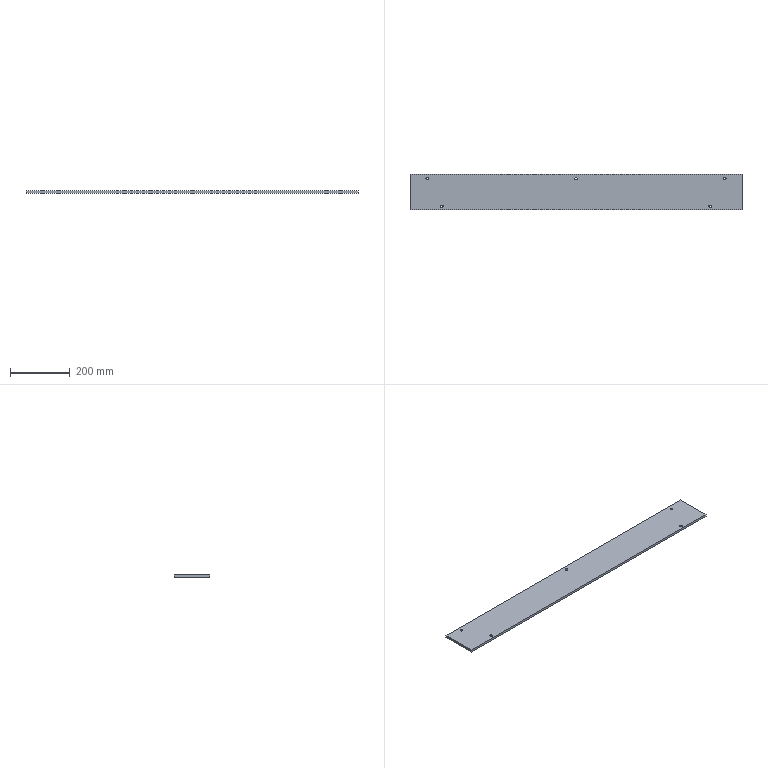Part | SolidWorks | features Extrusion 1, HoleWzd 1 | 1 solid | 16 faces | box 1116 x 120 x 8 mm | volume 1069090 mm3 | cylinder 10 | plane 6 | commonest cylinder face diameters 8.5 x10
STEP:
#1=CARTESIAN_POINT('',(-504.25,45.,0.));
#2=VERTEX_POINT('',#1);
#3=CARTESIAN_POINT('',(-495.75,45.,0.));
#4=VERTEX_POINT('',#3);
#5=CARTESIAN_POINT('',(-500.,45.,0.));
#6=DIRECTION('',(0.,0.,1.));
#7=DIRECTION('',(1.,0.,0.));
#8=AXIS2_PLACEMENT_3D('',#5,#6,#7);
#9=CIRCLE('',#8,4.25);
#10=EDGE_CURVE('',#2,#4,#9,.T.);
#11=ORIENTED_EDGE('',*,*,#10,.F.);
#12=CARTESIAN_POINT('',(-504.25,45.,8.));
#13=VERTEX_POINT('',#12);
#14=CARTESIAN_POINT('',(-504.25,45.,8.));
#15=DIRECTION('',(0.,0.,1.));
#16=VECTOR('',#15,1000.);
#17=LINE('',#14,#16);
#18=EDGE_CURVE('',#2,#13,#17,.T.);
#19=ORIENTED_EDGE('',*,*,#18,.T.);
#20=CARTESIAN_POINT('',(-495.75,45.,8.));
#21=VERTEX_POINT('',#20);
#22=CARTESIAN_POINT('',(-500.,45.,8.));
#23=DIRECTION('',(0.,0.,1.));
#24=DIRECTION('',(1.,0.,0.));
#25=AXIS2_PLACEMENT_3D('',#22,#23,#24);
#26=CIRCLE('',#25,4.25);
#27=EDGE_CURVE('',#13,#21,#26,.T.);
#28=ORIENTED_EDGE('',*,*,#27,.T.);
#29=CARTESIAN_POINT('',(-495.75,45.,8.));
#30=DIRECTION('',(0.,0.,1.));
#31=VECTOR('',#30,1000.);
#32=LINE('',#29,#31);
#33=EDGE_CURVE('',#4,#21,#32,.T.);
#34=ORIENTED_EDGE('',*,*,#33,.F.);
#35=EDGE_LOOP('',(#11,#19,#28,#34));
#36=FACE_OUTER_BOUND('',#35,.T.);
#37=CARTESIAN_POINT('',(-500.,45.,8.));
#38=DIRECTION('',(0.,0.,1.));
#39=DIRECTION('',(1.,0.,0.));
#40=AXIS2_PLACEMENT_3D('',#37,#38,#39);
#41=CYLINDRICAL_SURFACE('',#40,4.25);
#42=ADVANCED_FACE('',(#36),#41,.F.);
#43=CARTESIAN_POINT('',(-455.25,-48.,0.));
#44=VERTEX_POINT('',#43);
#45=CARTESIAN_POINT('',(-446.75,-48.,0.));
#46=VERTEX_POINT('',#45);
#47=CARTESIAN_POINT('',(-451.,-48.,0.));
#48=DIRECTION('',(0.,0.,1.));
#49=DIRECTION('',(1.,0.,0.));
#50=AXIS2_PLACEMENT_3D('',#47,#48,#49);
#51=CIRCLE('',#50,4.25);
#52=EDGE_CURVE('',#44,#46,#51,.T.);
#53=ORIENTED_EDGE('',*,*,#52,.F.);
#54=CARTESIAN_POINT('',(-455.25,-48.,8.));
#55=VERTEX_POINT('',#54);
#56=CARTESIAN_POINT('',(-455.25,-48.,8.));
#57=DIRECTION('',(0.,0.,1.));
#58=VECTOR('',#57,1000.);
#59=LINE('',#56,#58);
#60=EDGE_CURVE('',#44,#55,#59,.T.);
#61=ORIENTED_EDGE('',*,*,#60,.T.);
#62=CARTESIAN_POINT('',(-446.75,-48.,8.));
#63=VERTEX_POINT('',#62);
#64=CARTESIAN_POINT('',(-451.,-48.,8.));
#65=DIRECTION('',(0.,0.,1.));
#66=DIRECTION('',(1.,0.,0.));
#67=AXIS2_PLACEMENT_3D('',#64,#65,#66);
#68=CIRCLE('',#67,4.25);
#69=EDGE_CURVE('',#55,#63,#68,.T.);
#70=ORIENTED_EDGE('',*,*,#69,.T.);
#71=CARTESIAN_POINT('',(-446.75,-48.,8.));
#72=DIRECTION('',(0.,0.,1.));
#73=VECTOR('',#72,1000.);
#74=LINE('',#71,#73);
#75=EDGE_CURVE('',#46,#63,#74,.T.);
#76=ORIENTED_EDGE('',*,*,#75,.F.);
#77=EDGE_LOOP('',(#53,#61,#70,#76));
#78=FACE_OUTER_BOUND('',#77,.T.);
#79=CARTESIAN_POINT('',(-451.,-48.,8.));
#80=DIRECTION('',(0.,0.,1.));
#81=DIRECTION('',(1.,0.,0.));
#82=AXIS2_PLACEMENT_3D('',#79,#80,#81);
#83=CYLINDRICAL_SURFACE('',#82,4.25);
#84=ADVANCED_FACE('',(#78),#83,.F.);
#85=CARTESIAN_POINT('',(-4.25,45.,0.));
#86=VERTEX_POINT('',#85);
#87=CARTESIAN_POINT('',(4.25,45.,0.));
#88=VERTEX_POINT('',#87);
#89=CARTESIAN_POINT('',(0.,45.,0.));
#90=DIRECTION('',(0.,0.,1.));
#91=DIRECTION('',(1.,0.,0.));
#92=AXIS2_PLACEMENT_3D('',#89,#90,#91);
#93=CIRCLE('',#92,4.25);
#94=EDGE_CURVE('',#86,#88,#93,.T.);
#95=ORIENTED_EDGE('',*,*,#94,.F.);
#96=CARTESIAN_POINT('',(-4.25,45.,8.));
#97=VERTEX_POINT('',#96);
#98=CARTESIAN_POINT('',(-4.25,45.,8.));
#99=DIRECTION('',(0.,0.,1.));
#100=VECTOR('',#99,1000.);
#101=LINE('',#98,#100);
#102=EDGE_CURVE('',#86,#97,#101,.T.);
#103=ORIENTED_EDGE('',*,*,#102,.T.);
#104=CARTESIAN_POINT('',(4.25,45.,8.));
#105=VERTEX_POINT('',#104);
#106=CARTESIAN_POINT('',(0.,45.,8.));
#107=DIRECTION('',(0.,0.,1.));
#108=DIRECTION('',(1.,0.,0.));
#109=AXIS2_PLACEMENT_3D('',#106,#107,#108);
#110=CIRCLE('',#109,4.25);
#111=EDGE_CURVE('',#97,#105,#110,.T.);
#112=ORIENTED_EDGE('',*,*,#111,.T.);
#113=CARTESIAN_POINT('',(4.25,45.,8.));
#114=DIRECTION('',(0.,0.,1.));
#115=VECTOR('',#114,1000.);
#116=LINE('',#113,#115);
#117=EDGE_CURVE('',#88,#105,#116,.T.);
#118=ORIENTED_EDGE('',*,*,#117,.F.);
#119=EDGE_LOOP('',(#95,#103,#112,#118));
#120=FACE_OUTER_BOUND('',#119,.T.);
#121=CARTESIAN_POINT('',(0.,45.,8.));
#122=DIRECTION('',(0.,0.,1.));
#123=DIRECTION('',(1.,0.,0.));
#124=AXIS2_PLACEMENT_3D('',#121,#122,#123);
#125=CYLINDRICAL_SURFACE('',#124,4.25);
#126=ADVANCED_FACE('',(#120),#125,.F.);
#127=CARTESIAN_POINT('',(495.75,45.,0.));
#128=VERTEX_POINT('',#127);
#129=CARTESIAN_POINT('',(504.25,45.,0.));
#130=VERTEX_POINT('',#129);
#131=CARTESIAN_POINT('',(500.,45.,0.));
#132=DIRECTION('',(0.,0.,1.));
#133=DIRECTION('',(1.,0.,0.));
#134=AXIS2_PLACEMENT_3D('',#131,#132,#133);
#135=CIRCLE('',#134,4.25);
#136=EDGE_CURVE('',#128,#130,#135,.T.);
#137=ORIENTED_EDGE('',*,*,#136,.F.);
#138=CARTESIAN_POINT('',(495.75,45.,8.));
#139=VERTEX_POINT('',#138);
#140=CARTESIAN_POINT('',(495.75,45.,8.));
#141=DIRECTION('',(0.,0.,1.));
#142=VECTOR('',#141,1000.);
#143=LINE('',#140,#142);
#144=EDGE_CURVE('',#128,#139,#143,.T.);
#145=ORIENTED_EDGE('',*,*,#144,.T.);
#146=CARTESIAN_POINT('',(504.25,45.,8.));
#147=VERTEX_POINT('',#146);
#148=CARTESIAN_POINT('',(500.,45.,8.));
#149=DIRECTION('',(0.,0.,1.));
#150=DIRECTION('',(1.,0.,0.));
#151=AXIS2_PLACEMENT_3D('',#148,#149,#150);
#152=CIRCLE('',#151,4.25);
#153=EDGE_CURVE('',#139,#147,#152,.T.);
#154=ORIENTED_EDGE('',*,*,#153,.T.);
#155=CARTESIAN_POINT('',(504.25,45.,8.));
#156=DIRECTION('',(0.,0.,1.));
#157=VECTOR('',#156,1000.);
#158=LINE('',#155,#157);
#159=EDGE_CURVE('',#130,#147,#158,.T.);
#160=ORIENTED_EDGE('',*,*,#159,.F.);
#161=EDGE_LOOP('',(#137,#145,#154,#160));
#162=FACE_OUTER_BOUND('',#161,.T.);
#163=CARTESIAN_POINT('',(500.,45.,8.));
#164=DIRECTION('',(0.,0.,1.));
#165=DIRECTION('',(1.,0.,0.));
#166=AXIS2_PLACEMENT_3D('',#163,#164,#165);
#167=CYLINDRICAL_SURFACE('',#166,4.25);
#168=ADVANCED_FACE('',(#162),#167,.F.);
#169=CARTESIAN_POINT('',(446.75,-48.,0.));
#170=VERTEX_POINT('',#169);
#171=CARTESIAN_POINT('',(455.25,-48.,0.));
#172=VERTEX_POINT('',#171);
#173=CARTESIAN_POINT('',(451.,-48.,0.));
#174=DIRECTION('',(0.,0.,1.));
#175=DIRECTION('',(1.,0.,0.));
#176=AXIS2_PLACEMENT_3D('',#173,#174,#175);
#177=CIRCLE('',#176,4.25);
#178=EDGE_CURVE('',#170,#172,#177,.T.);
#179=ORIENTED_EDGE('',*,*,#178,.F.);
#180=CARTESIAN_POINT('',(446.75,-48.,8.));
#181=VERTEX_POINT('',#180);
#182=CARTESIAN_POINT('',(446.75,-48.,8.));
#183=DIRECTION('',(0.,0.,1.));
#184=VECTOR('',#183,1000.);
#185=LINE('',#182,#184);
#186=EDGE_CURVE('',#170,#181,#185,.T.);
#187=ORIENTED_EDGE('',*,*,#186,.T.);
#188=CARTESIAN_POINT('',(455.25,-48.,8.));
#189=VERTEX_POINT('',#188);
#190=CARTESIAN_POINT('',(451.,-48.,8.));
#191=DIRECTION('',(0.,0.,1.));
#192=DIRECTION('',(1.,0.,0.));
#193=AXIS2_PLACEMENT_3D('',#190,#191,#192);
#194=CIRCLE('',#193,4.25);
#195=EDGE_CURVE('',#181,#189,#194,.T.);
#196=ORIENTED_EDGE('',*,*,#195,.T.);
#197=CARTESIAN_POINT('',(455.25,-48.,8.));
#198=DIRECTION('',(0.,0.,1.));
#199=VECTOR('',#198,1000.);
#200=LINE('',#197,#199);
#201=EDGE_CURVE('',#172,#189,#200,.T.);
#202=ORIENTED_EDGE('',*,*,#201,.F.);
#203=EDGE_LOOP('',(#179,#187,#196,#202));
#204=FACE_OUTER_BOUND('',#203,.T.);
#205=CARTESIAN_POINT('',(451.,-48.,8.));
#206=DIRECTION('',(0.,0.,1.));
#207=DIRECTION('',(1.,0.,0.));
#208=AXIS2_PLACEMENT_3D('',#205,#206,#207);
#209=CYLINDRICAL_SURFACE('',#208,4.25);
#210=ADVANCED_FACE('',(#204),#209,.F.);
#211=CARTESIAN_POINT('',(558.,-60.,0.));
#212=VERTEX_POINT('',#211);
#213=CARTESIAN_POINT('',(558.,60.,0.));
#214=VERTEX_POINT('',#213);
#215=CARTESIAN_POINT('',(558.,60.,0.));
#216=DIRECTION('',(0.,1.,0.));
#217=VECTOR('',#216,1000.);
#218=LINE('',#215,#217);
#219=EDGE_CURVE('',#212,#214,#218,.T.);
#220=ORIENTED_EDGE('',*,*,#219,.T.);
#221=CARTESIAN_POINT('',(558.,60.,8.));
#222=VERTEX_POINT('',#221);
#223=CARTESIAN_POINT('',(558.,60.,8.));
#224=DIRECTION('',(0.,0.,-1.));
#225=VECTOR('',#224,1000.);
#226=LINE('',#223,#225);
#227=EDGE_CURVE('',#222,#214,#226,.T.);
#228=ORIENTED_EDGE('',*,*,#227,.F.);
#229=CARTESIAN_POINT('',(558.,-60.,8.));
#230=VERTEX_POINT('',#229);
#231=CARTESIAN_POINT('',(558.,60.,8.));
#232=DIRECTION('',(0.,1.,0.));
#233=VECTOR('',#232,1000.);
#234=LINE('',#231,#233);
#235=EDGE_CURVE('',#230,#222,#234,.T.);
#236=ORIENTED_EDGE('',*,*,#235,.F.);
#237=CARTESIAN_POINT('',(558.,-60.,8.));
#238=DIRECTION('',(0.,0.,-1.));
#239=VECTOR('',#238,1000.);
#240=LINE('',#237,#239);
#241=EDGE_CURVE('',#230,#212,#240,.T.);
#242=ORIENTED_EDGE('',*,*,#241,.T.);
#243=EDGE_LOOP('',(#220,#228,#236,#242));
#244=FACE_OUTER_BOUND('',#243,.T.);
#245=CARTESIAN_POINT('',(558.,60.,8.));
#246=DIRECTION('',(-1.,0.,0.));
#247=DIRECTION('',(0.,0.,1.));
#248=AXIS2_PLACEMENT_3D('',#245,#246,#247);
#249=PLANE('',#248);
#250=ADVANCED_FACE('',(#244),#249,.F.);
#251=CARTESIAN_POINT('',(-558.,60.,0.));
#252=VERTEX_POINT('',#251);
#253=CARTESIAN_POINT('',(-558.,60.,0.));
#254=DIRECTION('',(-1.,0.,0.));
#255=VECTOR('',#254,1000.);
#256=LINE('',#253,#255);
#257=EDGE_CURVE('',#214,#252,#256,.T.);
#258=ORIENTED_EDGE('',*,*,#257,.T.);
#259=CARTESIAN_POINT('',(-558.,60.,8.));
#260=VERTEX_POINT('',#259);
#261=CARTESIAN_POINT('',(-558.,60.,8.));
#262=DIRECTION('',(0.,0.,-1.));
#263=VECTOR('',#262,1000.);
#264=LINE('',#261,#263);
#265=EDGE_CURVE('',#260,#252,#264,.T.);
#266=ORIENTED_EDGE('',*,*,#265,.F.);
#267=CARTESIAN_POINT('',(-558.,60.,8.));
#268=DIRECTION('',(-1.,0.,0.));
#269=VECTOR('',#268,1000.);
#270=LINE('',#267,#269);
#271=EDGE_CURVE('',#222,#260,#270,.T.);
#272=ORIENTED_EDGE('',*,*,#271,.F.);
#273=ORIENTED_EDGE('',*,*,#227,.T.);
#274=EDGE_LOOP('',(#258,#266,#272,#273));
#275=FACE_OUTER_BOUND('',#274,.T.);
#276=CARTESIAN_POINT('',(-558.,60.,8.));
#277=DIRECTION('',(0.,-1.,0.));
#278=DIRECTION('',(0.,0.,-1.));
#279=AXIS2_PLACEMENT_3D('',#276,#277,#278);
#280=PLANE('',#279);
#281=ADVANCED_FACE('',(#275),#280,.F.);
#282=CARTESIAN_POINT('',(-558.,-60.,0.));
#283=VERTEX_POINT('',#282);
#284=CARTESIAN_POINT('',(-558.,60.,0.));
#285=DIRECTION('',(0.,-1.,0.));
#286=VECTOR('',#285,1000.);
#287=LINE('',#284,#286);
#288=EDGE_CURVE('',#252,#283,#287,.T.);
#289=ORIENTED_EDGE('',*,*,#288,.T.);
#290=CARTESIAN_POINT('',(-558.,-60.,8.));
#291=VERTEX_POINT('',#290);
#292=CARTESIAN_POINT('',(-558.,-60.,8.));
#293=DIRECTION('',(0.,0.,-1.));
#294=VECTOR('',#293,1000.);
#295=LINE('',#292,#294);
#296=EDGE_CURVE('',#291,#283,#295,.T.);
#297=ORIENTED_EDGE('',*,*,#296,.F.);
#298=CARTESIAN_POINT('',(-558.,60.,8.));
#299=DIRECTION('',(0.,-1.,0.));
#300=VECTOR('',#299,1000.);
#301=LINE('',#298,#300);
#302=EDGE_CURVE('',#260,#291,#301,.T.);
#303=ORIENTED_EDGE('',*,*,#302,.F.);
#304=ORIENTED_EDGE('',*,*,#265,.T.);
#305=EDGE_LOOP('',(#289,#297,#303,#304));
#306=FACE_OUTER_BOUND('',#305,.T.);
#307=CARTESIAN_POINT('',(-558.,60.,8.));
#308=DIRECTION('',(1.,0.,0.));
#309=DIRECTION('',(0.,0.,-1.));
#310=AXIS2_PLACEMENT_3D('',#307,#308,#309);
#311=PLANE('',#310);
#312=ADVANCED_FACE('',(#306),#311,.F.);
#313=CARTESIAN_POINT('',(-558.,-60.,0.));
#314=DIRECTION('',(1.,0.,0.));
#315=VECTOR('',#314,1000.);
#316=LINE('',#313,#315);
#317=EDGE_CURVE('',#283,#212,#316,.T.);
#318=ORIENTED_EDGE('',*,*,#317,.T.);
#319=ORIENTED_EDGE('',*,*,#241,.F.);
#320=CARTESIAN_POINT('',(-558.,-60.,8.));
#321=DIRECTION('',(1.,0.,0.));
#322=VECTOR('',#321,1000.);
#323=LINE('',#320,#322);
#324=EDGE_CURVE('',#291,#230,#323,.T.);
#325=ORIENTED_EDGE('',*,*,#324,.F.);
#326=ORIENTED_EDGE('',*,*,#296,.T.);
#327=EDGE_LOOP('',(#318,#319,#325,#326));
#328=FACE_OUTER_BOUND('',#327,.T.);
#329=CARTESIAN_POINT('',(-558.,-60.,8.));
#330=DIRECTION('',(0.,1.,0.));
#331=DIRECTION('',(0.,0.,1.));
#332=AXIS2_PLACEMENT_3D('',#329,#330,#331);
#333=PLANE('',#332);
#334=ADVANCED_FACE('',(#328),#333,.F.);
#335=CARTESIAN_POINT('',(-500.,45.,8.));
#336=DIRECTION('',(0.,0.,1.));
#337=DIRECTION('',(1.,0.,0.));
#338=AXIS2_PLACEMENT_3D('',#335,#336,#337);
#339=CIRCLE('',#338,4.25);
#340=EDGE_CURVE('',#21,#13,#339,.T.);
#341=ORIENTED_EDGE('',*,*,#340,.F.);
#342=ORIENTED_EDGE('',*,*,#27,.F.);
#343=EDGE_LOOP('',(#341,#342));
#344=FACE_BOUND('',#343,.T.);
#345=CARTESIAN_POINT('',(-451.,-48.,8.));
#346=DIRECTION('',(0.,0.,1.));
#347=DIRECTION('',(1.,0.,0.));
#348=AXIS2_PLACEMENT_3D('',#345,#346,#347);
#349=CIRCLE('',#348,4.25);
#350=EDGE_CURVE('',#63,#55,#349,.T.);
#351=ORIENTED_EDGE('',*,*,#350,.F.);
#352=ORIENTED_EDGE('',*,*,#69,.F.);
#353=EDGE_LOOP('',(#351,#352));
#354=FACE_BOUND('',#353,.T.);
#355=CARTESIAN_POINT('',(0.,45.,8.));
#356=DIRECTION('',(0.,0.,1.));
#357=DIRECTION('',(1.,0.,0.));
#358=AXIS2_PLACEMENT_3D('',#355,#356,#357);
#359=CIRCLE('',#358,4.25);
#360=EDGE_CURVE('',#105,#97,#359,.T.);
#361=ORIENTED_EDGE('',*,*,#360,.F.);
#362=ORIENTED_EDGE('',*,*,#111,.F.);
#363=EDGE_LOOP('',(#361,#362));
#364=FACE_BOUND('',#363,.T.);
#365=CARTESIAN_POINT('',(500.,45.,8.));
#366=DIRECTION('',(0.,0.,1.));
#367=DIRECTION('',(1.,0.,0.));
#368=AXIS2_PLACEMENT_3D('',#365,#366,#367);
#369=CIRCLE('',#368,4.25);
#370=EDGE_CURVE('',#147,#139,#369,.T.);
#371=ORIENTED_EDGE('',*,*,#370,.F.);
#372=ORIENTED_EDGE('',*,*,#153,.F.);
#373=EDGE_LOOP('',(#371,#372));
#374=FACE_BOUND('',#373,.T.);
#375=CARTESIAN_POINT('',(451.,-48.,8.));
#376=DIRECTION('',(0.,0.,1.));
#377=DIRECTION('',(1.,0.,0.));
#378=AXIS2_PLACEMENT_3D('',#375,#376,#377);
#379=CIRCLE('',#378,4.25);
#380=EDGE_CURVE('',#189,#181,#379,.T.);
#381=ORIENTED_EDGE('',*,*,#380,.F.);
#382=ORIENTED_EDGE('',*,*,#195,.F.);
#383=EDGE_LOOP('',(#381,#382));
#384=FACE_BOUND('',#383,.T.);
#385=ORIENTED_EDGE('',*,*,#235,.T.);
#386=ORIENTED_EDGE('',*,*,#271,.T.);
#387=ORIENTED_EDGE('',*,*,#302,.T.);
#388=ORIENTED_EDGE('',*,*,#324,.T.);
#389=EDGE_LOOP('',(#385,#386,#387,#388));
#390=FACE_OUTER_BOUND('',#389,.T.);
#391=CARTESIAN_POINT('',(0.,0.,8.));
#392=DIRECTION('',(0.,0.,1.));
#393=DIRECTION('',(1.,0.,0.));
#394=AXIS2_PLACEMENT_3D('',#391,#392,#393);
#395=PLANE('',#394);
#396=ADVANCED_FACE('',(#344,#354,#364,#374,#384,#390),#395,.T.);
#397=CARTESIAN_POINT('',(-500.,45.,0.));
#398=DIRECTION('',(0.,0.,1.));
#399=DIRECTION('',(1.,0.,0.));
#400=AXIS2_PLACEMENT_3D('',#397,#398,#399);
#401=CIRCLE('',#400,4.25);
#402=EDGE_CURVE('',#4,#2,#401,.T.);
#403=ORIENTED_EDGE('',*,*,#402,.T.);
#404=ORIENTED_EDGE('',*,*,#10,.T.);
#405=EDGE_LOOP('',(#403,#404));
#406=FACE_BOUND('',#405,.T.);
#407=CARTESIAN_POINT('',(-451.,-48.,0.));
#408=DIRECTION('',(0.,0.,1.));
#409=DIRECTION('',(1.,0.,0.));
#410=AXIS2_PLACEMENT_3D('',#407,#408,#409);
#411=CIRCLE('',#410,4.25);
#412=EDGE_CURVE('',#46,#44,#411,.T.);
#413=ORIENTED_EDGE('',*,*,#412,.T.);
#414=ORIENTED_EDGE('',*,*,#52,.T.);
#415=EDGE_LOOP('',(#413,#414));
#416=FACE_BOUND('',#415,.T.);
#417=CARTESIAN_POINT('',(0.,45.,0.));
#418=DIRECTION('',(0.,0.,1.));
#419=DIRECTION('',(1.,0.,0.));
#420=AXIS2_PLACEMENT_3D('',#417,#418,#419);
#421=CIRCLE('',#420,4.25);
#422=EDGE_CURVE('',#88,#86,#421,.T.);
#423=ORIENTED_EDGE('',*,*,#422,.T.);
#424=ORIENTED_EDGE('',*,*,#94,.T.);
#425=EDGE_LOOP('',(#423,#424));
#426=FACE_BOUND('',#425,.T.);
#427=CARTESIAN_POINT('',(500.,45.,0.));
#428=DIRECTION('',(0.,0.,1.));
#429=DIRECTION('',(1.,0.,0.));
#430=AXIS2_PLACEMENT_3D('',#427,#428,#429);
#431=CIRCLE('',#430,4.25);
#432=EDGE_CURVE('',#130,#128,#431,.T.);
#433=ORIENTED_EDGE('',*,*,#432,.T.);
#434=ORIENTED_EDGE('',*,*,#136,.T.);
#435=EDGE_LOOP('',(#433,#434));
#436=FACE_BOUND('',#435,.T.);
#437=CARTESIAN_POINT('',(451.,-48.,0.));
#438=DIRECTION('',(0.,0.,1.));
#439=DIRECTION('',(1.,0.,0.));
#440=AXIS2_PLACEMENT_3D('',#437,#438,#439);
#441=CIRCLE('',#440,4.25);
#442=EDGE_CURVE('',#172,#170,#441,.T.);
#443=ORIENTED_EDGE('',*,*,#442,.T.);
#444=ORIENTED_EDGE('',*,*,#178,.T.);
#445=EDGE_LOOP('',(#443,#444));
#446=FACE_BOUND('',#445,.T.);
#447=ORIENTED_EDGE('',*,*,#219,.F.);
#448=ORIENTED_EDGE('',*,*,#317,.F.);
#449=ORIENTED_EDGE('',*,*,#288,.F.);
#450=ORIENTED_EDGE('',*,*,#257,.F.);
#451=EDGE_LOOP('',(#447,#448,#449,#450));
#452=FACE_OUTER_BOUND('',#451,.T.);
#453=CARTESIAN_POINT('',(0.,0.,0.));
#454=DIRECTION('',(0.,0.,1.));
#455=DIRECTION('',(1.,0.,0.));
#456=AXIS2_PLACEMENT_3D('',#453,#454,#455);
#457=PLANE('',#456);
#458=ADVANCED_FACE('',(#406,#416,#426,#436,#446,#452),#457,.F.);
#459=ORIENTED_EDGE('',*,*,#186,.F.);
#460=ORIENTED_EDGE('',*,*,#442,.F.);
#461=ORIENTED_EDGE('',*,*,#201,.T.);
#462=ORIENTED_EDGE('',*,*,#380,.T.);
#463=EDGE_LOOP('',(#459,#460,#461,#462));
#464=FACE_OUTER_BOUND('',#463,.T.);
#465=CARTESIAN_POINT('',(451.,-48.,8.));
#466=DIRECTION('',(0.,0.,1.));
#467=DIRECTION('',(1.,0.,0.));
#468=AXIS2_PLACEMENT_3D('',#465,#466,#467);
#469=CYLINDRICAL_SURFACE('',#468,4.25);
#470=ADVANCED_FACE('',(#464),#469,.F.);
#471=ORIENTED_EDGE('',*,*,#144,.F.);
#472=ORIENTED_EDGE('',*,*,#432,.F.);
#473=ORIENTED_EDGE('',*,*,#159,.T.);
#474=ORIENTED_EDGE('',*,*,#370,.T.);
#475=EDGE_LOOP('',(#471,#472,#473,#474));
#476=FACE_OUTER_BOUND('',#475,.T.);
#477=CARTESIAN_POINT('',(500.,45.,8.));
#478=DIRECTION('',(0.,0.,1.));
#479=DIRECTION('',(1.,0.,0.));
#480=AXIS2_PLACEMENT_3D('',#477,#478,#479);
#481=CYLINDRICAL_SURFACE('',#480,4.25);
#482=ADVANCED_FACE('',(#476),#481,.F.);
#483=ORIENTED_EDGE('',*,*,#102,.F.);
#484=ORIENTED_EDGE('',*,*,#422,.F.);
#485=ORIENTED_EDGE('',*,*,#117,.T.);
#486=ORIENTED_EDGE('',*,*,#360,.T.);
#487=EDGE_LOOP('',(#483,#484,#485,#486));
#488=FACE_OUTER_BOUND('',#487,.T.);
#489=CARTESIAN_POINT('',(0.,45.,8.));
#490=DIRECTION('',(0.,0.,1.));
#491=DIRECTION('',(1.,0.,0.));
#492=AXIS2_PLACEMENT_3D('',#489,#490,#491);
#493=CYLINDRICAL_SURFACE('',#492,4.25);
#494=ADVANCED_FACE('',(#488),#493,.F.);
#495=ORIENTED_EDGE('',*,*,#60,.F.);
#496=ORIENTED_EDGE('',*,*,#412,.F.);
#497=ORIENTED_EDGE('',*,*,#75,.T.);
#498=ORIENTED_EDGE('',*,*,#350,.T.);
#499=EDGE_LOOP('',(#495,#496,#497,#498));
#500=FACE_OUTER_BOUND('',#499,.T.);
#501=CARTESIAN_POINT('',(-451.,-48.,8.));
#502=DIRECTION('',(0.,0.,1.));
#503=DIRECTION('',(1.,0.,0.));
#504=AXIS2_PLACEMENT_3D('',#501,#502,#503);
#505=CYLINDRICAL_SURFACE('',#504,4.25);
#506=ADVANCED_FACE('',(#500),#505,.F.);
#507=ORIENTED_EDGE('',*,*,#18,.F.);
#508=ORIENTED_EDGE('',*,*,#402,.F.);
#509=ORIENTED_EDGE('',*,*,#33,.T.);
#510=ORIENTED_EDGE('',*,*,#340,.T.);
#511=EDGE_LOOP('',(#507,#508,#509,#510));
#512=FACE_OUTER_BOUND('',#511,.T.);
#513=CARTESIAN_POINT('',(-500.,45.,8.));
#514=DIRECTION('',(0.,0.,1.));
#515=DIRECTION('',(1.,0.,0.));
#516=AXIS2_PLACEMENT_3D('',#513,#514,#515);
#517=CYLINDRICAL_SURFACE('',#516,4.25);
#518=ADVANCED_FACE('',(#512),#517,.F.);
#519=CLOSED_SHELL('',(#42,#84,#126,#168,#210,#250,#281,#312,#334,#396,#458,#470,#482,#494,#506,#518));
#520=MANIFOLD_SOLID_BREP('',#519);
#521=CARTESIAN_POINT('',(0.,0.,0.));
#522=DIRECTION('',(0.,0.,1.));
#523=DIRECTION('',(1.,0.,0.));
#524=AXIS2_PLACEMENT_3D('',#521,#522,#523);
#525=(LENGTH_UNIT()NAMED_UNIT(*)SI_UNIT(.MILLI.,.METRE.));
#526=UNCERTAINTY_MEASURE_WITH_UNIT(LENGTH_MEASURE(0.00001),#525,'','');
#527=(NAMED_UNIT(*)PLANE_ANGLE_UNIT()SI_UNIT($,.RADIAN.));
#528=(NAMED_UNIT(*)SI_UNIT($,.STERADIAN.)SOLID_ANGLE_UNIT());
#529=(GEOMETRIC_REPRESENTATION_CONTEXT(3)GLOBAL_UNCERTAINTY_ASSIGNED_CONTEXT((#526))GLOBAL_UNIT_ASSIGNED_CONTEXT((#525,#527,#528))REPRESENTATION_CONTEXT('',''));
#530=ADVANCED_BREP_SHAPE_REPRESENTATION('',(#520,#524),#529);